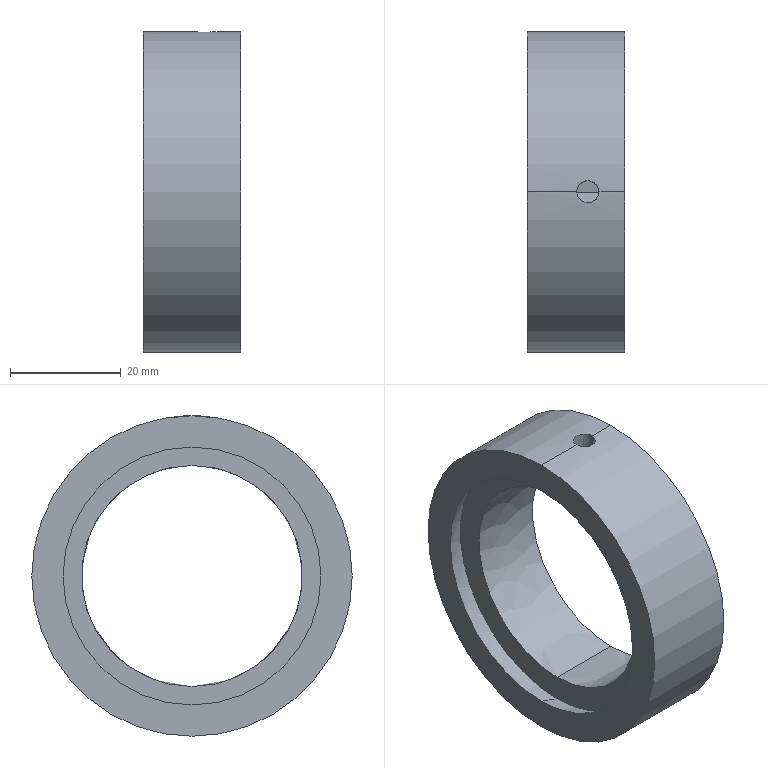Part | SolidWorks | features BaseBody 1 | 1 solid | 11 faces | box 17.7 x 58 x 58 mm | volume 22163 mm3 | spline 6 | plane 3 | cylinder 2 | commonest cylinder face diameters 58 x2
STEP:
#1=CARTESIAN_POINT('',(17.5,75.,25.875));
#2=VERTEX_POINT('',#1);
#3=CARTESIAN_POINT('',(17.5,75.,72.525));
#4=VERTEX_POINT('',#3);
#5=CARTESIAN_POINT('',(17.5,75.,49.2));
#6=DIRECTION('',(1.,0.,0.));
#7=DIRECTION('',(0.,0.,1.));
#8=AXIS2_PLACEMENT_3D('',#5,#6,#7);
#9=CIRCLE('',#8,23.325);
#10=EDGE_CURVE('',#2,#4,#9,.T.);
#11=ORIENTED_EDGE('',*,*,#10,.F.);
#12=CARTESIAN_POINT('',(21.5,75.,24.419));
#13=VERTEX_POINT('',#12);
#14=CARTESIAN_POINT('',(19.5,75.,25.147));
#15=DIRECTION('',(0.9397,0.,-0.342));
#16=VECTOR('',#15,1000.);
#17=LINE('',#14,#16);
#18=EDGE_CURVE('',#2,#13,#17,.T.);
#19=ORIENTED_EDGE('',*,*,#18,.T.);
#20=CARTESIAN_POINT('',(21.5,75.,73.981));
#21=VERTEX_POINT('',#20);
#22=CARTESIAN_POINT('',(21.5,75.,49.2));
#23=DIRECTION('',(1.,0.,0.));
#24=DIRECTION('',(0.,0.,1.));
#25=AXIS2_PLACEMENT_3D('',#22,#23,#24);
#26=CIRCLE('',#25,24.781);
#27=EDGE_CURVE('',#13,#21,#26,.T.);
#28=ORIENTED_EDGE('',*,*,#27,.T.);
#29=CARTESIAN_POINT('',(19.5,75.,73.253));
#30=DIRECTION('',(0.9397,0.,0.342));
#31=VECTOR('',#30,1000.);
#32=LINE('',#29,#31);
#33=EDGE_CURVE('',#4,#21,#32,.T.);
#34=ORIENTED_EDGE('',*,*,#33,.F.);
#35=EDGE_LOOP('',(#11,#19,#28,#34));
#36=FACE_OUTER_BOUND('',#35,.T.);
#37=CARTESIAN_POINT('',(17.5,75.,25.875));
#38=CARTESIAN_POINT('',(17.5,121.65,25.875));
#39=CARTESIAN_POINT('',(17.5,121.65,72.525));
#40=CARTESIAN_POINT('',(17.5,75.,72.525));
#41=CARTESIAN_POINT('',(21.5,75.,24.419));
#42=CARTESIAN_POINT('',(21.5,124.562,24.419));
#43=CARTESIAN_POINT('',(21.5,124.562,73.981));
#44=CARTESIAN_POINT('',(21.5,75.,73.981));
#45=(BOUNDED_SURFACE()B_SPLINE_SURFACE(1,3,((#37,#38,#39,#40),(#41,#42,#43,#44)),.UNSPECIFIED.,.F.,.F.,.F.)B_SPLINE_SURFACE_WITH_KNOTS((2,2),(4,4),(0.,1.),(0.,1.),.UNSPECIFIED.)GEOMETRIC_REPRESENTATION_ITEM()RATIONAL_B_SPLINE_SURFACE(((1.,0.3333,0.3333,1.),(1.,0.3333,0.3333,1.)))REPRESENTATION_ITEM('')SURFACE());
#46=ADVANCED_FACE('',(#36),#45,.T.);
#47=CARTESIAN_POINT('',(26.5,75.,78.2));
#48=VERTEX_POINT('',#47);
#49=CARTESIAN_POINT('',(30.5,75.,78.2));
#50=VERTEX_POINT('',#49);
#51=CARTESIAN_POINT('',(26.5,75.,78.2));
#52=CARTESIAN_POINT('',(26.5,75.132,78.2));
#53=CARTESIAN_POINT('',(26.513,75.262,78.199));
#54=CARTESIAN_POINT('',(26.564,75.518,78.196));
#55=CARTESIAN_POINT('',(26.602,75.645,78.193));
#56=CARTESIAN_POINT('',(26.703,75.887,78.187));
#57=CARTESIAN_POINT('',(26.764,76.002,78.183));
#58=CARTESIAN_POINT('',(26.909,76.219,78.175));
#59=CARTESIAN_POINT('',(26.994,76.322,78.17));
#60=CARTESIAN_POINT('',(27.27,76.599,78.156));
#61=CARTESIAN_POINT('',(27.493,76.748,78.147));
#62=CARTESIAN_POINT('',(27.974,76.947,78.135));
#63=CARTESIAN_POINT('',(28.238,77.,78.131));
#64=CARTESIAN_POINT('',(28.629,77.,78.131));
#65=CARTESIAN_POINT('',(28.762,76.987,78.132));
#66=CARTESIAN_POINT('',(29.018,76.936,78.135));
#67=CARTESIAN_POINT('',(29.143,76.898,78.138));
#68=CARTESIAN_POINT('',(29.385,76.798,78.144));
#69=CARTESIAN_POINT('',(29.502,76.736,78.148));
#70=CARTESIAN_POINT('',(29.719,76.591,78.156));
#71=CARTESIAN_POINT('',(29.82,76.508,78.161));
#72=CARTESIAN_POINT('',(30.007,76.322,78.17));
#73=CARTESIAN_POINT('',(30.089,76.221,78.174));
#74=CARTESIAN_POINT('',(30.234,76.004,78.183));
#75=CARTESIAN_POINT('',(30.297,75.888,78.187));
#76=CARTESIAN_POINT('',(30.398,75.645,78.193));
#77=CARTESIAN_POINT('',(30.435,75.521,78.196));
#78=CARTESIAN_POINT('',(30.487,75.264,78.199));
#79=CARTESIAN_POINT('',(30.5,75.132,78.2));
#80=CARTESIAN_POINT('',(30.5,75.,78.2));
#81=B_SPLINE_CURVE_WITH_KNOTS('',3,(#51,#52,#53,#54,#55,#56,#57,#58,#59,#60,#61,#62,#63,#64,#65,#66,#67,#68,#69,#70,#71,#72,#73,#74,#75,#76,#77,#78,#79,#80),.UNSPECIFIED.,.F.,.F.,(4,2,2,2,2,2,2,2,2,2,2,2,2,2,4),(0.,0.0003908,0.0007817,0.001173,0.001563,0.002345,0.003127,0.003518,0.003908,0.004299,0.00469,0.005081,0.005472,0.005863,0.006253),.UNSPECIFIED.);
#82=EDGE_CURVE('',#48,#50,#81,.T.);
#83=ORIENTED_EDGE('',*,*,#82,.F.);
#84=CARTESIAN_POINT('',(26.5,75.,69.2));
#85=VERTEX_POINT('',#84);
#86=CARTESIAN_POINT('',(26.5,75.,73.));
#87=DIRECTION('',(0.,0.,-1.));
#88=VECTOR('',#87,1000.);
#89=LINE('',#86,#88);
#90=EDGE_CURVE('',#48,#85,#89,.T.);
#91=ORIENTED_EDGE('',*,*,#90,.T.);
#92=CARTESIAN_POINT('',(30.5,75.,69.2));
#93=VERTEX_POINT('',#92);
#94=CARTESIAN_POINT('',(30.5,75.,69.2));
#95=CARTESIAN_POINT('',(30.5,75.132,69.2));
#96=CARTESIAN_POINT('',(30.487,75.262,69.199));
#97=CARTESIAN_POINT('',(30.436,75.518,69.194));
#98=CARTESIAN_POINT('',(30.398,75.645,69.19));
#99=CARTESIAN_POINT('',(30.297,75.887,69.181));
#100=CARTESIAN_POINT('',(30.236,76.001,69.175));
#101=CARTESIAN_POINT('',(30.091,76.219,69.163));
#102=CARTESIAN_POINT('',(30.007,76.322,69.157));
#103=CARTESIAN_POINT('',(29.73,76.598,69.137));
#104=CARTESIAN_POINT('',(29.508,76.747,69.124));
#105=CARTESIAN_POINT('',(29.027,76.947,69.105));
#106=CARTESIAN_POINT('',(28.764,77.,69.1));
#107=CARTESIAN_POINT('',(28.368,77.,69.1));
#108=CARTESIAN_POINT('',(28.238,76.987,69.101));
#109=CARTESIAN_POINT('',(27.982,76.936,69.106));
#110=CARTESIAN_POINT('',(27.855,76.898,69.11));
#111=CARTESIAN_POINT('',(27.613,76.797,69.119));
#112=CARTESIAN_POINT('',(27.499,76.736,69.125));
#113=CARTESIAN_POINT('',(27.281,76.591,69.137));
#114=CARTESIAN_POINT('',(27.178,76.507,69.143));
#115=CARTESIAN_POINT('',(26.902,76.23,69.163));
#116=CARTESIAN_POINT('',(26.753,76.008,69.176));
#117=CARTESIAN_POINT('',(26.553,75.527,69.195));
#118=CARTESIAN_POINT('',(26.5,75.264,69.2));
#119=CARTESIAN_POINT('',(26.5,75.,69.2));
#120=B_SPLINE_CURVE_WITH_KNOTS('',3,(#94,#95,#96,#97,#98,#99,#100,#101,#102,#103,#104,#105,#106,#107,#108,#109,#110,#111,#112,#113,#114,#115,#116,#117,#118,#119),.UNSPECIFIED.,.F.,.F.,(4,2,2,2,2,2,2,2,2,2,2,2,4),(0.009382,0.009773,0.01016,0.01055,0.01094,0.01173,0.01251,0.0129,0.01329,0.01368,0.01407,0.01485,0.01563),.UNSPECIFIED.);
#121=EDGE_CURVE('',#93,#85,#120,.T.);
#122=ORIENTED_EDGE('',*,*,#121,.F.);
#123=CARTESIAN_POINT('',(30.5,75.,73.));
#124=DIRECTION('',(0.,0.,-1.));
#125=VECTOR('',#124,1000.);
#126=LINE('',#123,#125);
#127=EDGE_CURVE('',#50,#93,#126,.T.);
#128=ORIENTED_EDGE('',*,*,#127,.F.);
#129=EDGE_LOOP('',(#83,#91,#122,#128));
#130=FACE_OUTER_BOUND('',#129,.T.);
#131=CARTESIAN_POINT('',(30.5,75.,78.255));
#132=CARTESIAN_POINT('',(30.5,75.,69.045));
#133=CARTESIAN_POINT('',(30.5,79.,78.255));
#134=CARTESIAN_POINT('',(30.5,79.,69.045));
#135=CARTESIAN_POINT('',(26.5,79.,78.255));
#136=CARTESIAN_POINT('',(26.5,79.,69.045));
#137=CARTESIAN_POINT('',(26.5,75.,78.255));
#138=CARTESIAN_POINT('',(26.5,75.,69.045));
#139=(BOUNDED_SURFACE()B_SPLINE_SURFACE(3,1,((#131,#132),(#133,#134),(#135,#136),(#137,#138)),.UNSPECIFIED.,.F.,.F.,.F.)B_SPLINE_SURFACE_WITH_KNOTS((4,4),(2,2),(0.,1.),(0.,1.),.UNSPECIFIED.)GEOMETRIC_REPRESENTATION_ITEM()RATIONAL_B_SPLINE_SURFACE(((1.,1.),(0.3333,0.3333),(0.3333,0.3333),(1.,1.)))REPRESENTATION_ITEM('')SURFACE());
#140=ADVANCED_FACE('',(#130),#139,.T.);
#141=CARTESIAN_POINT('',(21.5,75.,29.2));
#142=VERTEX_POINT('',#141);
#143=CARTESIAN_POINT('',(21.5,75.,69.2));
#144=VERTEX_POINT('',#143);
#145=CARTESIAN_POINT('',(21.5,75.,49.2));
#146=DIRECTION('',(1.,0.,0.));
#147=DIRECTION('',(0.,0.,1.));
#148=AXIS2_PLACEMENT_3D('',#145,#146,#147);
#149=CIRCLE('',#148,20.);
#150=EDGE_CURVE('',#142,#144,#149,.T.);
#151=ORIENTED_EDGE('',*,*,#150,.F.);
#152=CARTESIAN_POINT('',(35.2,75.,29.2));
#153=VERTEX_POINT('',#152);
#154=CARTESIAN_POINT('',(28.35,75.,29.2));
#155=DIRECTION('',(1.,0.,0.));
#156=VECTOR('',#155,1000.);
#157=LINE('',#154,#156);
#158=EDGE_CURVE('',#142,#153,#157,.T.);
#159=ORIENTED_EDGE('',*,*,#158,.T.);
#160=CARTESIAN_POINT('',(35.2,75.,69.2));
#161=VERTEX_POINT('',#160);
#162=CARTESIAN_POINT('',(35.2,75.,49.2));
#163=DIRECTION('',(1.,0.,0.));
#164=DIRECTION('',(0.,0.,1.));
#165=AXIS2_PLACEMENT_3D('',#162,#163,#164);
#166=CIRCLE('',#165,20.);
#167=EDGE_CURVE('',#153,#161,#166,.T.);
#168=ORIENTED_EDGE('',*,*,#167,.T.);
#169=CARTESIAN_POINT('',(28.35,75.,69.2));
#170=DIRECTION('',(1.,0.,0.));
#171=VECTOR('',#170,1000.);
#172=LINE('',#169,#171);
#173=EDGE_CURVE('',#93,#161,#172,.T.);
#174=ORIENTED_EDGE('',*,*,#173,.F.);
#175=ORIENTED_EDGE('',*,*,#121,.T.);
#176=CARTESIAN_POINT('',(28.35,75.,69.2));
#177=DIRECTION('',(1.,0.,0.));
#178=VECTOR('',#177,1000.);
#179=LINE('',#176,#178);
#180=EDGE_CURVE('',#144,#85,#179,.T.);
#181=ORIENTED_EDGE('',*,*,#180,.F.);
#182=EDGE_LOOP('',(#151,#159,#168,#174,#175,#181));
#183=FACE_OUTER_BOUND('',#182,.T.);
#184=CARTESIAN_POINT('',(21.5,75.,69.2));
#185=CARTESIAN_POINT('',(35.2,75.,69.2));
#186=CARTESIAN_POINT('',(21.5,115.,69.2));
#187=CARTESIAN_POINT('',(35.2,115.,69.2));
#188=CARTESIAN_POINT('',(21.5,115.,29.2));
#189=CARTESIAN_POINT('',(35.2,115.,29.2));
#190=CARTESIAN_POINT('',(21.5,75.,29.2));
#191=CARTESIAN_POINT('',(35.2,75.,29.2));
#192=(BOUNDED_SURFACE()B_SPLINE_SURFACE(3,1,((#184,#185),(#186,#187),(#188,#189),(#190,#191)),.UNSPECIFIED.,.F.,.F.,.F.)B_SPLINE_SURFACE_WITH_KNOTS((4,4),(2,2),(0.,1.),(0.,1.),.UNSPECIFIED.)GEOMETRIC_REPRESENTATION_ITEM()RATIONAL_B_SPLINE_SURFACE(((1.,1.),(0.3333,0.3333),(0.3333,0.3333),(1.,1.)))REPRESENTATION_ITEM('')SURFACE());
#193=ADVANCED_FACE('',(#183),#192,.T.);
#194=CARTESIAN_POINT('',(17.5,75.,20.2));
#195=VERTEX_POINT('',#194);
#196=CARTESIAN_POINT('',(17.5,75.,78.2));
#197=VERTEX_POINT('',#196);
#198=CARTESIAN_POINT('',(17.5,75.,49.2));
#199=DIRECTION('',(1.,0.,0.));
#200=DIRECTION('',(0.,0.,1.));
#201=AXIS2_PLACEMENT_3D('',#198,#199,#200);
#202=CIRCLE('',#201,29.);
#203=EDGE_CURVE('',#195,#197,#202,.T.);
#204=ORIENTED_EDGE('',*,*,#203,.T.);
#205=CARTESIAN_POINT('',(26.35,75.,78.2));
#206=DIRECTION('',(1.,0.,0.));
#207=VECTOR('',#206,1000.);
#208=LINE('',#205,#207);
#209=EDGE_CURVE('',#197,#48,#208,.T.);
#210=ORIENTED_EDGE('',*,*,#209,.T.);
#211=ORIENTED_EDGE('',*,*,#82,.T.);
#212=CARTESIAN_POINT('',(35.2,75.,78.2));
#213=VERTEX_POINT('',#212);
#214=CARTESIAN_POINT('',(26.35,75.,78.2));
#215=DIRECTION('',(1.,0.,0.));
#216=VECTOR('',#215,1000.);
#217=LINE('',#214,#216);
#218=EDGE_CURVE('',#50,#213,#217,.T.);
#219=ORIENTED_EDGE('',*,*,#218,.T.);
#220=CARTESIAN_POINT('',(35.2,75.,20.2));
#221=VERTEX_POINT('',#220);
#222=CARTESIAN_POINT('',(35.2,75.,49.2));
#223=DIRECTION('',(1.,0.,0.));
#224=DIRECTION('',(0.,0.,1.));
#225=AXIS2_PLACEMENT_3D('',#222,#223,#224);
#226=CIRCLE('',#225,29.);
#227=EDGE_CURVE('',#221,#213,#226,.T.);
#228=ORIENTED_EDGE('',*,*,#227,.F.);
#229=CARTESIAN_POINT('',(26.35,75.,20.2));
#230=DIRECTION('',(1.,0.,0.));
#231=VECTOR('',#230,1000.);
#232=LINE('',#229,#231);
#233=EDGE_CURVE('',#195,#221,#232,.T.);
#234=ORIENTED_EDGE('',*,*,#233,.F.);
#235=EDGE_LOOP('',(#204,#210,#211,#219,#228,#234));
#236=FACE_OUTER_BOUND('',#235,.T.);
#237=CARTESIAN_POINT('',(26.35,75.,49.2));
#238=DIRECTION('',(1.,0.,0.));
#239=DIRECTION('',(0.,0.,-1.));
#240=AXIS2_PLACEMENT_3D('',#237,#238,#239);
#241=CYLINDRICAL_SURFACE('',#240,29.);
#242=ADVANCED_FACE('',(#236),#241,.T.);
#243=ORIENTED_EDGE('',*,*,#227,.T.);
#244=CARTESIAN_POINT('',(35.2,75.,49.2));
#245=DIRECTION('',(1.,0.,0.));
#246=DIRECTION('',(0.,0.,1.));
#247=AXIS2_PLACEMENT_3D('',#244,#245,#246);
#248=CIRCLE('',#247,29.);
#249=EDGE_CURVE('',#213,#221,#248,.T.);
#250=ORIENTED_EDGE('',*,*,#249,.T.);
#251=EDGE_LOOP('',(#243,#250));
#252=FACE_OUTER_BOUND('',#251,.T.);
#253=CARTESIAN_POINT('',(35.2,75.,49.2));
#254=DIRECTION('',(1.,0.,0.));
#255=DIRECTION('',(0.,0.,1.));
#256=AXIS2_PLACEMENT_3D('',#253,#254,#255);
#257=CIRCLE('',#256,20.);
#258=EDGE_CURVE('',#161,#153,#257,.T.);
#259=ORIENTED_EDGE('',*,*,#258,.F.);
#260=ORIENTED_EDGE('',*,*,#167,.F.);
#261=EDGE_LOOP('',(#259,#260));
#262=FACE_BOUND('',#261,.T.);
#263=CARTESIAN_POINT('',(35.2,75.,73.7));
#264=DIRECTION('',(1.,0.,0.));
#265=DIRECTION('',(0.,0.,-1.));
#266=AXIS2_PLACEMENT_3D('',#263,#264,#265);
#267=PLANE('',#266);
#268=ADVANCED_FACE('',(#252,#262),#267,.T.);
#269=ORIENTED_EDGE('',*,*,#209,.F.);
#270=CARTESIAN_POINT('',(17.5,75.,49.2));
#271=DIRECTION('',(1.,0.,0.));
#272=DIRECTION('',(0.,0.,1.));
#273=AXIS2_PLACEMENT_3D('',#270,#271,#272);
#274=CIRCLE('',#273,29.);
#275=EDGE_CURVE('',#197,#195,#274,.T.);
#276=ORIENTED_EDGE('',*,*,#275,.T.);
#277=ORIENTED_EDGE('',*,*,#233,.T.);
#278=ORIENTED_EDGE('',*,*,#249,.F.);
#279=ORIENTED_EDGE('',*,*,#218,.F.);
#280=CARTESIAN_POINT('',(30.5,75.,78.2));
#281=CARTESIAN_POINT('',(30.5,74.868,78.2));
#282=CARTESIAN_POINT('',(30.487,74.738,78.199));
#283=CARTESIAN_POINT('',(30.436,74.482,78.196));
#284=CARTESIAN_POINT('',(30.398,74.355,78.193));
#285=CARTESIAN_POINT('',(30.297,74.113,78.187));
#286=CARTESIAN_POINT('',(30.236,73.998,78.183));
#287=CARTESIAN_POINT('',(30.091,73.781,78.175));
#288=CARTESIAN_POINT('',(30.006,73.678,78.17));
#289=CARTESIAN_POINT('',(29.73,73.401,78.156));
#290=CARTESIAN_POINT('',(29.507,73.252,78.147));
#291=CARTESIAN_POINT('',(29.026,73.053,78.135));
#292=CARTESIAN_POINT('',(28.762,73.,78.131));
#293=CARTESIAN_POINT('',(28.371,73.,78.131));
#294=CARTESIAN_POINT('',(28.238,73.013,78.132));
#295=CARTESIAN_POINT('',(27.982,73.064,78.135));
#296=CARTESIAN_POINT('',(27.857,73.102,78.138));
#297=CARTESIAN_POINT('',(27.615,73.202,78.144));
#298=CARTESIAN_POINT('',(27.498,73.264,78.148));
#299=CARTESIAN_POINT('',(27.281,73.409,78.156));
#300=CARTESIAN_POINT('',(27.18,73.492,78.161));
#301=CARTESIAN_POINT('',(26.993,73.678,78.17));
#302=CARTESIAN_POINT('',(26.911,73.779,78.174));
#303=CARTESIAN_POINT('',(26.766,73.996,78.183));
#304=CARTESIAN_POINT('',(26.703,74.112,78.187));
#305=CARTESIAN_POINT('',(26.602,74.355,78.193));
#306=CARTESIAN_POINT('',(26.565,74.479,78.196));
#307=CARTESIAN_POINT('',(26.513,74.736,78.199));
#308=CARTESIAN_POINT('',(26.5,74.868,78.2));
#309=CARTESIAN_POINT('',(26.5,75.,78.2));
#310=B_SPLINE_CURVE_WITH_KNOTS('',3,(#280,#281,#282,#283,#284,#285,#286,#287,#288,#289,#290,#291,#292,#293,#294,#295,#296,#297,#298,#299,#300,#301,#302,#303,#304,#305,#306,#307,#308,#309),.UNSPECIFIED.,.F.,.F.,(4,2,2,2,2,2,2,2,2,2,2,2,2,2,4),(0.006253,0.006644,0.007035,0.007426,0.007817,0.008598,0.00938,0.009771,0.01016,0.01055,0.01094,0.01133,0.01173,0.01212,0.01251),.UNSPECIFIED.);
#311=EDGE_CURVE('',#50,#48,#310,.T.);
#312=ORIENTED_EDGE('',*,*,#311,.T.);
#313=EDGE_LOOP('',(#269,#276,#277,#278,#279,#312));
#314=FACE_OUTER_BOUND('',#313,.T.);
#315=CARTESIAN_POINT('',(26.35,75.,49.2));
#316=DIRECTION('',(1.,0.,0.));
#317=DIRECTION('',(0.,0.,-1.));
#318=AXIS2_PLACEMENT_3D('',#315,#316,#317);
#319=CYLINDRICAL_SURFACE('',#318,29.);
#320=ADVANCED_FACE('',(#314),#319,.T.);
#321=CARTESIAN_POINT('',(17.5,75.,49.2));
#322=DIRECTION('',(1.,0.,0.));
#323=DIRECTION('',(0.,0.,1.));
#324=AXIS2_PLACEMENT_3D('',#321,#322,#323);
#325=CIRCLE('',#324,23.325);
#326=EDGE_CURVE('',#4,#2,#325,.T.);
#327=ORIENTED_EDGE('',*,*,#326,.T.);
#328=ORIENTED_EDGE('',*,*,#10,.T.);
#329=EDGE_LOOP('',(#327,#328));
#330=FACE_BOUND('',#329,.T.);
#331=ORIENTED_EDGE('',*,*,#203,.F.);
#332=ORIENTED_EDGE('',*,*,#275,.F.);
#333=EDGE_LOOP('',(#331,#332));
#334=FACE_OUTER_BOUND('',#333,.T.);
#335=CARTESIAN_POINT('',(17.5,75.,75.363));
#336=DIRECTION('',(-1.,0.,0.));
#337=DIRECTION('',(0.,0.,1.));
#338=AXIS2_PLACEMENT_3D('',#335,#336,#337);
#339=PLANE('',#338);
#340=ADVANCED_FACE('',(#330,#334),#339,.T.);
#341=ORIENTED_EDGE('',*,*,#18,.F.);
#342=ORIENTED_EDGE('',*,*,#326,.F.);
#343=ORIENTED_EDGE('',*,*,#33,.T.);
#344=CARTESIAN_POINT('',(21.5,75.,49.2));
#345=DIRECTION('',(1.,0.,0.));
#346=DIRECTION('',(0.,0.,1.));
#347=AXIS2_PLACEMENT_3D('',#344,#345,#346);
#348=CIRCLE('',#347,24.781);
#349=EDGE_CURVE('',#21,#13,#348,.T.);
#350=ORIENTED_EDGE('',*,*,#349,.T.);
#351=EDGE_LOOP('',(#341,#342,#343,#350));
#352=FACE_OUTER_BOUND('',#351,.T.);
#353=CARTESIAN_POINT('',(17.5,75.,72.525));
#354=CARTESIAN_POINT('',(17.5,28.35,72.525));
#355=CARTESIAN_POINT('',(17.5,28.35,25.875));
#356=CARTESIAN_POINT('',(17.5,75.,25.875));
#357=CARTESIAN_POINT('',(21.5,75.,73.981));
#358=CARTESIAN_POINT('',(21.5,25.438,73.981));
#359=CARTESIAN_POINT('',(21.5,25.438,24.419));
#360=CARTESIAN_POINT('',(21.5,75.,24.419));
#361=(BOUNDED_SURFACE()B_SPLINE_SURFACE(1,3,((#353,#354,#355,#356),(#357,#358,#359,#360)),.UNSPECIFIED.,.F.,.F.,.F.)B_SPLINE_SURFACE_WITH_KNOTS((2,2),(4,4),(0.,1.),(0.,1.),.UNSPECIFIED.)GEOMETRIC_REPRESENTATION_ITEM()RATIONAL_B_SPLINE_SURFACE(((1.,0.3333,0.3333,1.),(1.,0.3333,0.3333,1.)))REPRESENTATION_ITEM('')SURFACE());
#362=ADVANCED_FACE('',(#352),#361,.T.);
#363=CARTESIAN_POINT('',(21.5,75.,49.2));
#364=DIRECTION('',(1.,0.,0.));
#365=DIRECTION('',(0.,0.,1.));
#366=AXIS2_PLACEMENT_3D('',#363,#364,#365);
#367=CIRCLE('',#366,20.);
#368=EDGE_CURVE('',#144,#142,#367,.T.);
#369=ORIENTED_EDGE('',*,*,#368,.T.);
#370=ORIENTED_EDGE('',*,*,#150,.T.);
#371=EDGE_LOOP('',(#369,#370));
#372=FACE_BOUND('',#371,.T.);
#373=ORIENTED_EDGE('',*,*,#349,.F.);
#374=ORIENTED_EDGE('',*,*,#27,.F.);
#375=EDGE_LOOP('',(#373,#374));
#376=FACE_OUTER_BOUND('',#375,.T.);
#377=CARTESIAN_POINT('',(21.5,75.,71.59));
#378=DIRECTION('',(-1.,0.,0.));
#379=DIRECTION('',(0.,0.,1.));
#380=AXIS2_PLACEMENT_3D('',#377,#378,#379);
#381=PLANE('',#380);
#382=ADVANCED_FACE('',(#372,#376),#381,.T.);
#383=ORIENTED_EDGE('',*,*,#158,.F.);
#384=ORIENTED_EDGE('',*,*,#368,.F.);
#385=ORIENTED_EDGE('',*,*,#180,.T.);
#386=CARTESIAN_POINT('',(26.5,75.,69.2));
#387=CARTESIAN_POINT('',(26.5,74.868,69.2));
#388=CARTESIAN_POINT('',(26.513,74.738,69.199));
#389=CARTESIAN_POINT('',(26.564,74.482,69.194));
#390=CARTESIAN_POINT('',(26.602,74.355,69.19));
#391=CARTESIAN_POINT('',(26.703,74.113,69.181));
#392=CARTESIAN_POINT('',(26.764,73.998,69.175));
#393=CARTESIAN_POINT('',(26.909,73.781,69.163));
#394=CARTESIAN_POINT('',(26.994,73.678,69.156));
#395=CARTESIAN_POINT('',(27.27,73.401,69.137));
#396=CARTESIAN_POINT('',(27.493,73.252,69.124));
#397=CARTESIAN_POINT('',(27.974,73.053,69.105));
#398=CARTESIAN_POINT('',(28.238,73.,69.1));
#399=CARTESIAN_POINT('',(28.629,73.,69.1));
#400=CARTESIAN_POINT('',(28.762,73.013,69.101));
#401=CARTESIAN_POINT('',(29.018,73.064,69.106));
#402=CARTESIAN_POINT('',(29.143,73.102,69.11));
#403=CARTESIAN_POINT('',(29.385,73.202,69.119));
#404=CARTESIAN_POINT('',(29.502,73.264,69.125));
#405=CARTESIAN_POINT('',(29.719,73.409,69.137));
#406=CARTESIAN_POINT('',(29.82,73.492,69.143));
#407=CARTESIAN_POINT('',(30.007,73.678,69.156));
#408=CARTESIAN_POINT('',(30.089,73.779,69.163));
#409=CARTESIAN_POINT('',(30.234,73.995,69.175));
#410=CARTESIAN_POINT('',(30.297,74.112,69.181));
#411=CARTESIAN_POINT('',(30.397,74.354,69.19));
#412=CARTESIAN_POINT('',(30.435,74.479,69.194));
#413=CARTESIAN_POINT('',(30.487,74.735,69.199));
#414=CARTESIAN_POINT('',(30.5,74.868,69.2));
#415=CARTESIAN_POINT('',(30.5,75.,69.2));
#416=B_SPLINE_CURVE_WITH_KNOTS('',3,(#386,#387,#388,#389,#390,#391,#392,#393,#394,#395,#396,#397,#398,#399,#400,#401,#402,#403,#404,#405,#406,#407,#408,#409,#410,#411,#412,#413,#414,#415),.UNSPECIFIED.,.F.,.F.,(4,2,2,2,2,2,2,2,2,2,2,2,2,2,4),(0.003126,0.003517,0.003908,0.004299,0.00469,0.005472,0.006254,0.006645,0.007036,0.007427,0.007818,0.008209,0.0086,0.008991,0.009382),.UNSPECIFIED.);
#417=EDGE_CURVE('',#85,#93,#416,.T.);
#418=ORIENTED_EDGE('',*,*,#417,.T.);
#419=ORIENTED_EDGE('',*,*,#173,.T.);
#420=ORIENTED_EDGE('',*,*,#258,.T.);
#421=EDGE_LOOP('',(#383,#384,#385,#418,#419,#420));
#422=FACE_OUTER_BOUND('',#421,.T.);
#423=CARTESIAN_POINT('',(21.5,75.,29.2));
#424=CARTESIAN_POINT('',(35.2,75.,29.2));
#425=CARTESIAN_POINT('',(21.5,35.,29.2));
#426=CARTESIAN_POINT('',(35.2,35.,29.2));
#427=CARTESIAN_POINT('',(21.5,35.,69.2));
#428=CARTESIAN_POINT('',(35.2,35.,69.2));
#429=CARTESIAN_POINT('',(21.5,75.,69.2));
#430=CARTESIAN_POINT('',(35.2,75.,69.2));
#431=(BOUNDED_SURFACE()B_SPLINE_SURFACE(3,1,((#423,#424),(#425,#426),(#427,#428),(#429,#430)),.UNSPECIFIED.,.F.,.F.,.T.)B_SPLINE_SURFACE_WITH_KNOTS((4,4),(2,2),(0.,1.),(0.,1.),.UNSPECIFIED.)GEOMETRIC_REPRESENTATION_ITEM()RATIONAL_B_SPLINE_SURFACE(((1.,1.),(0.3333,0.3333),(0.3333,0.3333),(1.,1.)))REPRESENTATION_ITEM('')SURFACE());
#432=ADVANCED_FACE('',(#422),#431,.T.);
#433=ORIENTED_EDGE('',*,*,#90,.F.);
#434=ORIENTED_EDGE('',*,*,#311,.F.);
#435=ORIENTED_EDGE('',*,*,#127,.T.);
#436=ORIENTED_EDGE('',*,*,#417,.F.);
#437=EDGE_LOOP('',(#433,#434,#435,#436));
#438=FACE_OUTER_BOUND('',#437,.T.);
#439=CARTESIAN_POINT('',(26.5,75.,78.255));
#440=CARTESIAN_POINT('',(26.5,75.,69.044));
#441=CARTESIAN_POINT('',(26.5,71.,78.255));
#442=CARTESIAN_POINT('',(26.5,71.,69.044));
#443=CARTESIAN_POINT('',(30.5,71.,78.255));
#444=CARTESIAN_POINT('',(30.5,71.,69.044));
#445=CARTESIAN_POINT('',(30.5,75.,78.255));
#446=CARTESIAN_POINT('',(30.5,75.,69.044));
#447=(BOUNDED_SURFACE()B_SPLINE_SURFACE(3,1,((#439,#440),(#441,#442),(#443,#444),(#445,#446)),.UNSPECIFIED.,.F.,.F.,.F.)B_SPLINE_SURFACE_WITH_KNOTS((4,4),(2,2),(0.,1.),(0.,1.),.UNSPECIFIED.)GEOMETRIC_REPRESENTATION_ITEM()RATIONAL_B_SPLINE_SURFACE(((1.,1.),(0.3333,0.3333),(0.3333,0.3333),(1.,1.)))REPRESENTATION_ITEM('')SURFACE());
#448=ADVANCED_FACE('',(#438),#447,.T.);
#449=CLOSED_SHELL('',(#46,#140,#193,#242,#268,#320,#340,#362,#382,#432,#448));
#450=MANIFOLD_SOLID_BREP('',#449);
#451=CARTESIAN_POINT('',(0.,0.,0.));
#452=DIRECTION('',(0.,0.,1.));
#453=DIRECTION('',(1.,0.,0.));
#454=AXIS2_PLACEMENT_3D('',#451,#452,#453);
#455=(LENGTH_UNIT()NAMED_UNIT(*)SI_UNIT(.MILLI.,.METRE.));
#456=UNCERTAINTY_MEASURE_WITH_UNIT(LENGTH_MEASURE(0.00001),#455,'','');
#457=(NAMED_UNIT(*)PLANE_ANGLE_UNIT()SI_UNIT($,.RADIAN.));
#458=(NAMED_UNIT(*)SI_UNIT($,.STERADIAN.)SOLID_ANGLE_UNIT());
#459=(GEOMETRIC_REPRESENTATION_CONTEXT(3)GLOBAL_UNCERTAINTY_ASSIGNED_CONTEXT((#456))GLOBAL_UNIT_ASSIGNED_CONTEXT((#455,#457,#458))REPRESENTATION_CONTEXT('',''));
#460=ADVANCED_BREP_SHAPE_REPRESENTATION('',(#450,#454),#459);